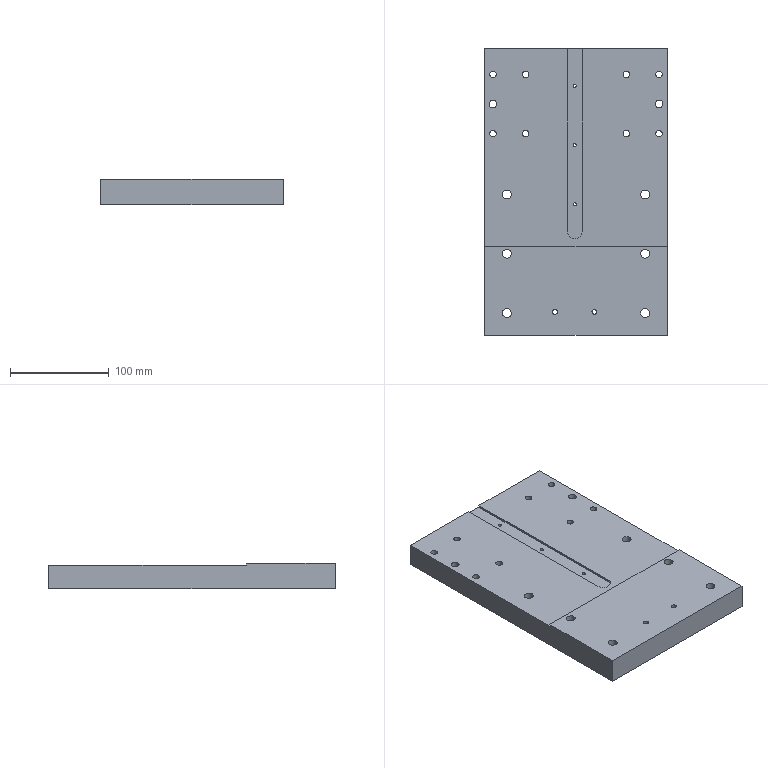Part | STEP file | SN10_006_007_PLACA | 1 solid | 33 faces | box 185 x 290 x 25.5 mm | volume 1268482 mm3 | cylinder 22 | plane 11 | commonest cylinder face diameters 6.647 x8 9 x6 3.242 x3 4.917 x2 8 x2 15 x1